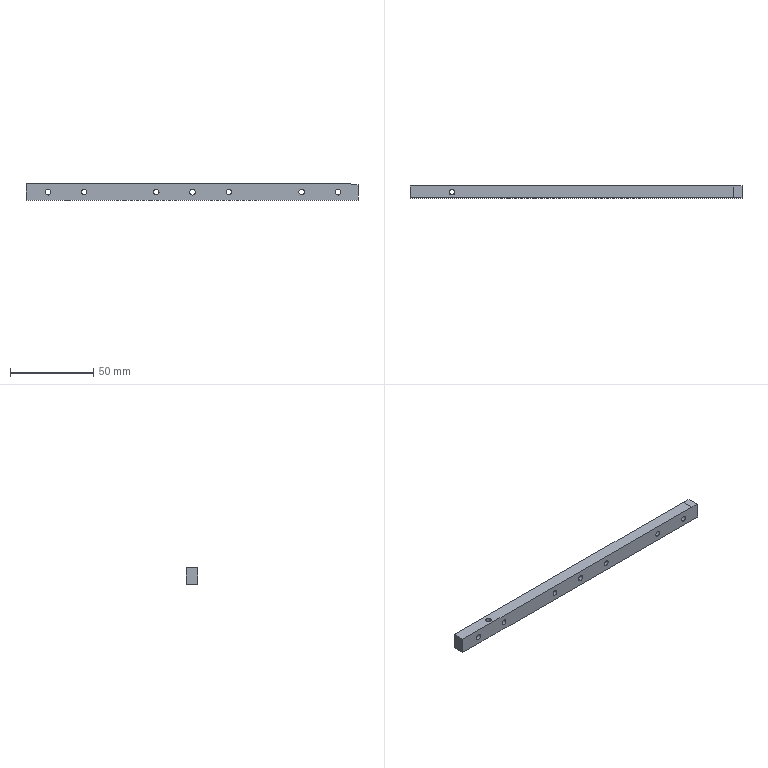Part | NX | 1 solid | 48 faces | box 199.5 x 7.2 x 9.8 mm | volume 13264 mm3 | cylinder 24 | cone 14 | plane 10 | commonest cylinder face diameters 3.3 x8 3.5 x6 6 x6 2.5 x2 3 x2